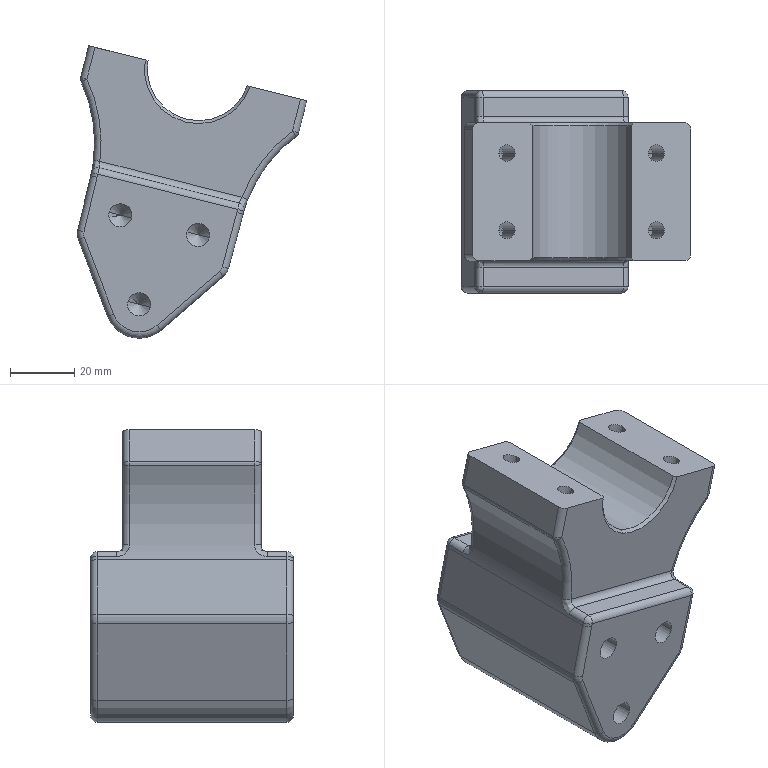Part | SolidWorks | features BaseBody 1 | 1 solid | 113 faces | box 71.4 x 63 x 91.099 mm | volume 188204 mm3 | cylinder 49 | cone 23 | torus 15 | plane 14 | sphere 8 | spline 4 | commonest cylinder face diameters 4 x22 7.2 x12 5.2 x8 10 x2 21.093 x2 88.833 x2